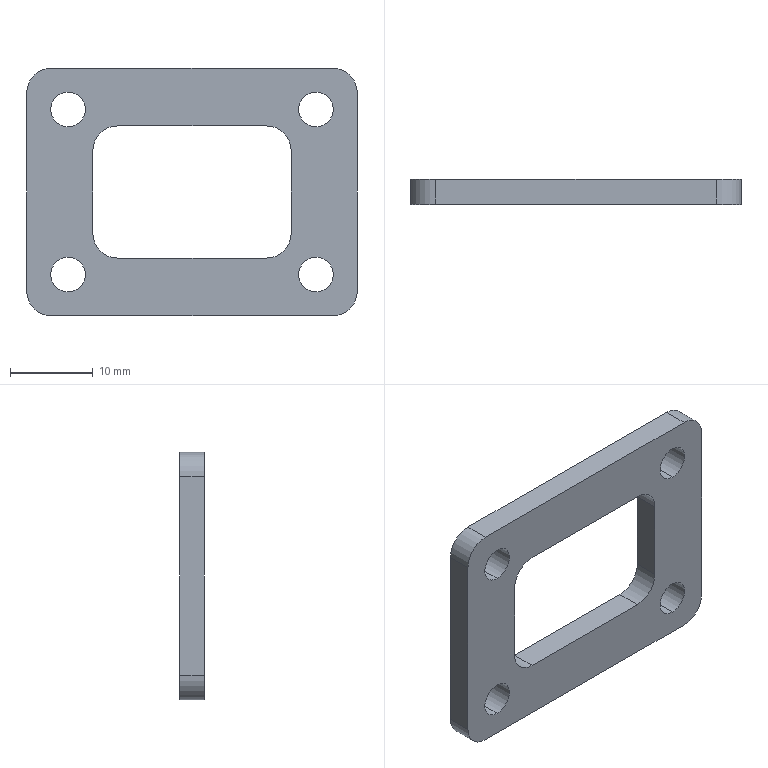Part | SolidWorks | features Extrusion 1 | 1 solid | 26 faces | box 40 x 3 x 30 mm | volume 2282 mm3 | cylinder 16 | plane 10 | commonest cylinder face diameters 4.2 x8 6 x8
STEP:
#1=CARTESIAN_POINT('',(15.,3.,7.9));
#2=VERTEX_POINT('',#1);
#3=CARTESIAN_POINT('',(15.,3.,12.1));
#4=VERTEX_POINT('',#3);
#5=CARTESIAN_POINT('',(15.,3.,10.));
#6=DIRECTION('',(0.,1.,0.));
#7=DIRECTION('',(0.,0.,1.));
#8=AXIS2_PLACEMENT_3D('',#5,#6,#7);
#9=CIRCLE('',#8,2.1);
#10=EDGE_CURVE('',#2,#4,#9,.T.);
#11=ORIENTED_EDGE('',*,*,#10,.T.);
#12=CARTESIAN_POINT('',(15.,0.,12.1));
#13=VERTEX_POINT('',#12);
#14=CARTESIAN_POINT('',(15.,3.,12.1));
#15=DIRECTION('',(0.,-1.,0.));
#16=VECTOR('',#15,1000.);
#17=LINE('',#14,#16);
#18=EDGE_CURVE('',#4,#13,#17,.T.);
#19=ORIENTED_EDGE('',*,*,#18,.T.);
#20=CARTESIAN_POINT('',(15.,0.,7.9));
#21=VERTEX_POINT('',#20);
#22=CARTESIAN_POINT('',(15.,0.,10.));
#23=DIRECTION('',(0.,1.,0.));
#24=DIRECTION('',(0.,0.,1.));
#25=AXIS2_PLACEMENT_3D('',#22,#23,#24);
#26=CIRCLE('',#25,2.1);
#27=EDGE_CURVE('',#21,#13,#26,.T.);
#28=ORIENTED_EDGE('',*,*,#27,.F.);
#29=CARTESIAN_POINT('',(15.,3.,7.9));
#30=DIRECTION('',(0.,-1.,0.));
#31=VECTOR('',#30,1000.);
#32=LINE('',#29,#31);
#33=EDGE_CURVE('',#2,#21,#32,.T.);
#34=ORIENTED_EDGE('',*,*,#33,.F.);
#35=EDGE_LOOP('',(#11,#19,#28,#34));
#36=FACE_OUTER_BOUND('',#35,.T.);
#37=CARTESIAN_POINT('',(15.,3.,10.));
#38=DIRECTION('',(0.,-1.,0.));
#39=DIRECTION('',(0.,0.,-1.));
#40=AXIS2_PLACEMENT_3D('',#37,#38,#39);
#41=CYLINDRICAL_SURFACE('',#40,2.1);
#42=ADVANCED_FACE('',(#36),#41,.F.);
#43=CARTESIAN_POINT('',(-15.,3.,7.9));
#44=VERTEX_POINT('',#43);
#45=CARTESIAN_POINT('',(-15.,3.,12.1));
#46=VERTEX_POINT('',#45);
#47=CARTESIAN_POINT('',(-15.,3.,10.));
#48=DIRECTION('',(0.,1.,0.));
#49=DIRECTION('',(0.,0.,1.));
#50=AXIS2_PLACEMENT_3D('',#47,#48,#49);
#51=CIRCLE('',#50,2.1);
#52=EDGE_CURVE('',#44,#46,#51,.T.);
#53=ORIENTED_EDGE('',*,*,#52,.T.);
#54=CARTESIAN_POINT('',(-15.,0.,12.1));
#55=VERTEX_POINT('',#54);
#56=CARTESIAN_POINT('',(-15.,3.,12.1));
#57=DIRECTION('',(0.,-1.,0.));
#58=VECTOR('',#57,1000.);
#59=LINE('',#56,#58);
#60=EDGE_CURVE('',#46,#55,#59,.T.);
#61=ORIENTED_EDGE('',*,*,#60,.T.);
#62=CARTESIAN_POINT('',(-15.,0.,7.9));
#63=VERTEX_POINT('',#62);
#64=CARTESIAN_POINT('',(-15.,0.,10.));
#65=DIRECTION('',(0.,1.,0.));
#66=DIRECTION('',(0.,0.,1.));
#67=AXIS2_PLACEMENT_3D('',#64,#65,#66);
#68=CIRCLE('',#67,2.1);
#69=EDGE_CURVE('',#63,#55,#68,.T.);
#70=ORIENTED_EDGE('',*,*,#69,.F.);
#71=CARTESIAN_POINT('',(-15.,3.,7.9));
#72=DIRECTION('',(0.,-1.,0.));
#73=VECTOR('',#72,1000.);
#74=LINE('',#71,#73);
#75=EDGE_CURVE('',#44,#63,#74,.T.);
#76=ORIENTED_EDGE('',*,*,#75,.F.);
#77=EDGE_LOOP('',(#53,#61,#70,#76));
#78=FACE_OUTER_BOUND('',#77,.T.);
#79=CARTESIAN_POINT('',(-15.,3.,10.));
#80=DIRECTION('',(0.,-1.,0.));
#81=DIRECTION('',(0.,0.,-1.));
#82=AXIS2_PLACEMENT_3D('',#79,#80,#81);
#83=CYLINDRICAL_SURFACE('',#82,2.1);
#84=ADVANCED_FACE('',(#78),#83,.F.);
#85=CARTESIAN_POINT('',(15.,3.,-12.1));
#86=VERTEX_POINT('',#85);
#87=CARTESIAN_POINT('',(15.,3.,-7.9));
#88=VERTEX_POINT('',#87);
#89=CARTESIAN_POINT('',(15.,3.,-10.));
#90=DIRECTION('',(0.,1.,0.));
#91=DIRECTION('',(0.,0.,1.));
#92=AXIS2_PLACEMENT_3D('',#89,#90,#91);
#93=CIRCLE('',#92,2.1);
#94=EDGE_CURVE('',#86,#88,#93,.T.);
#95=ORIENTED_EDGE('',*,*,#94,.T.);
#96=CARTESIAN_POINT('',(15.,0.,-7.9));
#97=VERTEX_POINT('',#96);
#98=CARTESIAN_POINT('',(15.,3.,-7.9));
#99=DIRECTION('',(0.,-1.,0.));
#100=VECTOR('',#99,1000.);
#101=LINE('',#98,#100);
#102=EDGE_CURVE('',#88,#97,#101,.T.);
#103=ORIENTED_EDGE('',*,*,#102,.T.);
#104=CARTESIAN_POINT('',(15.,0.,-12.1));
#105=VERTEX_POINT('',#104);
#106=CARTESIAN_POINT('',(15.,0.,-10.));
#107=DIRECTION('',(0.,1.,0.));
#108=DIRECTION('',(0.,0.,1.));
#109=AXIS2_PLACEMENT_3D('',#106,#107,#108);
#110=CIRCLE('',#109,2.1);
#111=EDGE_CURVE('',#105,#97,#110,.T.);
#112=ORIENTED_EDGE('',*,*,#111,.F.);
#113=CARTESIAN_POINT('',(15.,3.,-12.1));
#114=DIRECTION('',(0.,-1.,0.));
#115=VECTOR('',#114,1000.);
#116=LINE('',#113,#115);
#117=EDGE_CURVE('',#86,#105,#116,.T.);
#118=ORIENTED_EDGE('',*,*,#117,.F.);
#119=EDGE_LOOP('',(#95,#103,#112,#118));
#120=FACE_OUTER_BOUND('',#119,.T.);
#121=CARTESIAN_POINT('',(15.,3.,-10.));
#122=DIRECTION('',(0.,-1.,0.));
#123=DIRECTION('',(0.,0.,-1.));
#124=AXIS2_PLACEMENT_3D('',#121,#122,#123);
#125=CYLINDRICAL_SURFACE('',#124,2.1);
#126=ADVANCED_FACE('',(#120),#125,.F.);
#127=CARTESIAN_POINT('',(-15.,3.,-12.1));
#128=VERTEX_POINT('',#127);
#129=CARTESIAN_POINT('',(-15.,3.,-7.9));
#130=VERTEX_POINT('',#129);
#131=CARTESIAN_POINT('',(-15.,3.,-10.));
#132=DIRECTION('',(0.,1.,0.));
#133=DIRECTION('',(0.,0.,1.));
#134=AXIS2_PLACEMENT_3D('',#131,#132,#133);
#135=CIRCLE('',#134,2.1);
#136=EDGE_CURVE('',#128,#130,#135,.T.);
#137=ORIENTED_EDGE('',*,*,#136,.T.);
#138=CARTESIAN_POINT('',(-15.,0.,-7.9));
#139=VERTEX_POINT('',#138);
#140=CARTESIAN_POINT('',(-15.,3.,-7.9));
#141=DIRECTION('',(0.,-1.,0.));
#142=VECTOR('',#141,1000.);
#143=LINE('',#140,#142);
#144=EDGE_CURVE('',#130,#139,#143,.T.);
#145=ORIENTED_EDGE('',*,*,#144,.T.);
#146=CARTESIAN_POINT('',(-15.,0.,-12.1));
#147=VERTEX_POINT('',#146);
#148=CARTESIAN_POINT('',(-15.,0.,-10.));
#149=DIRECTION('',(0.,1.,0.));
#150=DIRECTION('',(0.,0.,1.));
#151=AXIS2_PLACEMENT_3D('',#148,#149,#150);
#152=CIRCLE('',#151,2.1);
#153=EDGE_CURVE('',#147,#139,#152,.T.);
#154=ORIENTED_EDGE('',*,*,#153,.F.);
#155=CARTESIAN_POINT('',(-15.,3.,-12.1));
#156=DIRECTION('',(0.,-1.,0.));
#157=VECTOR('',#156,1000.);
#158=LINE('',#155,#157);
#159=EDGE_CURVE('',#128,#147,#158,.T.);
#160=ORIENTED_EDGE('',*,*,#159,.F.);
#161=EDGE_LOOP('',(#137,#145,#154,#160));
#162=FACE_OUTER_BOUND('',#161,.T.);
#163=CARTESIAN_POINT('',(-15.,3.,-10.));
#164=DIRECTION('',(0.,-1.,0.));
#165=DIRECTION('',(0.,0.,-1.));
#166=AXIS2_PLACEMENT_3D('',#163,#164,#165);
#167=CYLINDRICAL_SURFACE('',#166,2.1);
#168=ADVANCED_FACE('',(#162),#167,.F.);
#169=ORIENTED_EDGE('',*,*,#52,.F.);
#170=CARTESIAN_POINT('',(-15.,3.,10.));
#171=DIRECTION('',(0.,1.,0.));
#172=DIRECTION('',(0.,0.,1.));
#173=AXIS2_PLACEMENT_3D('',#170,#171,#172);
#174=CIRCLE('',#173,2.1);
#175=EDGE_CURVE('',#46,#44,#174,.T.);
#176=ORIENTED_EDGE('',*,*,#175,.F.);
#177=EDGE_LOOP('',(#169,#176));
#178=FACE_BOUND('',#177,.T.);
#179=ORIENTED_EDGE('',*,*,#136,.F.);
#180=CARTESIAN_POINT('',(-15.,3.,-10.));
#181=DIRECTION('',(0.,1.,0.));
#182=DIRECTION('',(0.,0.,1.));
#183=AXIS2_PLACEMENT_3D('',#180,#181,#182);
#184=CIRCLE('',#183,2.1);
#185=EDGE_CURVE('',#130,#128,#184,.T.);
#186=ORIENTED_EDGE('',*,*,#185,.F.);
#187=EDGE_LOOP('',(#179,#186));
#188=FACE_BOUND('',#187,.T.);
#189=CARTESIAN_POINT('',(17.,3.,15.));
#190=VERTEX_POINT('',#189);
#191=CARTESIAN_POINT('',(20.,3.,12.));
#192=VERTEX_POINT('',#191);
#193=CARTESIAN_POINT('',(17.,3.,12.));
#194=DIRECTION('',(0.,1.,0.));
#195=DIRECTION('',(0.,0.,1.));
#196=AXIS2_PLACEMENT_3D('',#193,#194,#195);
#197=CIRCLE('',#196,3.);
#198=EDGE_CURVE('',#190,#192,#197,.T.);
#199=ORIENTED_EDGE('',*,*,#198,.T.);
#200=CARTESIAN_POINT('',(20.,3.,-12.));
#201=VERTEX_POINT('',#200);
#202=CARTESIAN_POINT('',(20.,3.,12.));
#203=DIRECTION('',(0.,0.,-1.));
#204=VECTOR('',#203,1000.);
#205=LINE('',#202,#204);
#206=EDGE_CURVE('',#192,#201,#205,.T.);
#207=ORIENTED_EDGE('',*,*,#206,.T.);
#208=CARTESIAN_POINT('',(17.,3.,-15.));
#209=VERTEX_POINT('',#208);
#210=CARTESIAN_POINT('',(17.,3.,-12.));
#211=DIRECTION('',(0.,1.,0.));
#212=DIRECTION('',(0.,0.,-1.));
#213=AXIS2_PLACEMENT_3D('',#210,#211,#212);
#214=CIRCLE('',#213,3.);
#215=EDGE_CURVE('',#201,#209,#214,.T.);
#216=ORIENTED_EDGE('',*,*,#215,.T.);
#217=CARTESIAN_POINT('',(-17.,3.,-15.));
#218=VERTEX_POINT('',#217);
#219=CARTESIAN_POINT('',(-17.,3.,-15.));
#220=DIRECTION('',(-1.,0.,0.));
#221=VECTOR('',#220,1000.);
#222=LINE('',#219,#221);
#223=EDGE_CURVE('',#209,#218,#222,.T.);
#224=ORIENTED_EDGE('',*,*,#223,.T.);
#225=CARTESIAN_POINT('',(-20.,3.,-12.));
#226=VERTEX_POINT('',#225);
#227=CARTESIAN_POINT('',(-17.,3.,-12.));
#228=DIRECTION('',(0.,1.,0.));
#229=DIRECTION('',(0.,0.,-1.));
#230=AXIS2_PLACEMENT_3D('',#227,#228,#229);
#231=CIRCLE('',#230,3.);
#232=EDGE_CURVE('',#218,#226,#231,.T.);
#233=ORIENTED_EDGE('',*,*,#232,.T.);
#234=CARTESIAN_POINT('',(-20.,3.,12.));
#235=VERTEX_POINT('',#234);
#236=CARTESIAN_POINT('',(-20.,3.,12.));
#237=DIRECTION('',(0.,0.,1.));
#238=VECTOR('',#237,1000.);
#239=LINE('',#236,#238);
#240=EDGE_CURVE('',#226,#235,#239,.T.);
#241=ORIENTED_EDGE('',*,*,#240,.T.);
#242=CARTESIAN_POINT('',(-17.,3.,15.));
#243=VERTEX_POINT('',#242);
#244=CARTESIAN_POINT('',(-17.,3.,12.));
#245=DIRECTION('',(0.,1.,0.));
#246=DIRECTION('',(0.,0.,-1.));
#247=AXIS2_PLACEMENT_3D('',#244,#245,#246);
#248=CIRCLE('',#247,3.);
#249=EDGE_CURVE('',#235,#243,#248,.T.);
#250=ORIENTED_EDGE('',*,*,#249,.T.);
#251=CARTESIAN_POINT('',(-17.,3.,15.));
#252=DIRECTION('',(1.,0.,0.));
#253=VECTOR('',#252,1000.);
#254=LINE('',#251,#253);
#255=EDGE_CURVE('',#243,#190,#254,.T.);
#256=ORIENTED_EDGE('',*,*,#255,.T.);
#257=EDGE_LOOP('',(#199,#207,#216,#224,#233,#241,#250,#256));
#258=FACE_OUTER_BOUND('',#257,.T.);
#259=ORIENTED_EDGE('',*,*,#94,.F.);
#260=CARTESIAN_POINT('',(15.,3.,-10.));
#261=DIRECTION('',(0.,1.,0.));
#262=DIRECTION('',(0.,0.,1.));
#263=AXIS2_PLACEMENT_3D('',#260,#261,#262);
#264=CIRCLE('',#263,2.1);
#265=EDGE_CURVE('',#88,#86,#264,.T.);
#266=ORIENTED_EDGE('',*,*,#265,.F.);
#267=EDGE_LOOP('',(#259,#266));
#268=FACE_BOUND('',#267,.T.);
#269=ORIENTED_EDGE('',*,*,#10,.F.);
#270=CARTESIAN_POINT('',(15.,3.,10.));
#271=DIRECTION('',(0.,1.,0.));
#272=DIRECTION('',(0.,0.,1.));
#273=AXIS2_PLACEMENT_3D('',#270,#271,#272);
#274=CIRCLE('',#273,2.1);
#275=EDGE_CURVE('',#4,#2,#274,.T.);
#276=ORIENTED_EDGE('',*,*,#275,.F.);
#277=EDGE_LOOP('',(#269,#276));
#278=FACE_BOUND('',#277,.T.);
#279=CARTESIAN_POINT('',(12.,3.,5.));
#280=VERTEX_POINT('',#279);
#281=CARTESIAN_POINT('',(12.,3.,-5.));
#282=VERTEX_POINT('',#281);
#283=CARTESIAN_POINT('',(12.,3.,5.));
#284=DIRECTION('',(0.,0.,-1.));
#285=VECTOR('',#284,1000.);
#286=LINE('',#283,#285);
#287=EDGE_CURVE('',#280,#282,#286,.T.);
#288=ORIENTED_EDGE('',*,*,#287,.F.);
#289=CARTESIAN_POINT('',(9.,3.,8.));
#290=VERTEX_POINT('',#289);
#291=CARTESIAN_POINT('',(9.,3.,5.));
#292=DIRECTION('',(0.,1.,0.));
#293=DIRECTION('',(0.,0.,1.));
#294=AXIS2_PLACEMENT_3D('',#291,#292,#293);
#295=CIRCLE('',#294,3.);
#296=EDGE_CURVE('',#290,#280,#295,.T.);
#297=ORIENTED_EDGE('',*,*,#296,.F.);
#298=CARTESIAN_POINT('',(-9.,3.,8.));
#299=VERTEX_POINT('',#298);
#300=CARTESIAN_POINT('',(-9.,3.,8.));
#301=DIRECTION('',(1.,0.,0.));
#302=VECTOR('',#301,1000.);
#303=LINE('',#300,#302);
#304=EDGE_CURVE('',#299,#290,#303,.T.);
#305=ORIENTED_EDGE('',*,*,#304,.F.);
#306=CARTESIAN_POINT('',(-12.,3.,5.));
#307=VERTEX_POINT('',#306);
#308=CARTESIAN_POINT('',(-9.,3.,5.));
#309=DIRECTION('',(0.,1.,0.));
#310=DIRECTION('',(0.,0.,-1.));
#311=AXIS2_PLACEMENT_3D('',#308,#309,#310);
#312=CIRCLE('',#311,3.);
#313=EDGE_CURVE('',#307,#299,#312,.T.);
#314=ORIENTED_EDGE('',*,*,#313,.F.);
#315=CARTESIAN_POINT('',(-12.,3.,-5.));
#316=VERTEX_POINT('',#315);
#317=CARTESIAN_POINT('',(-12.,3.,5.));
#318=DIRECTION('',(0.,0.,1.));
#319=VECTOR('',#318,1000.);
#320=LINE('',#317,#319);
#321=EDGE_CURVE('',#316,#307,#320,.T.);
#322=ORIENTED_EDGE('',*,*,#321,.F.);
#323=CARTESIAN_POINT('',(-9.,3.,-8.));
#324=VERTEX_POINT('',#323);
#325=CARTESIAN_POINT('',(-9.,3.,-5.));
#326=DIRECTION('',(0.,1.,0.));
#327=DIRECTION('',(0.,0.,-1.));
#328=AXIS2_PLACEMENT_3D('',#325,#326,#327);
#329=CIRCLE('',#328,3.);
#330=EDGE_CURVE('',#324,#316,#329,.T.);
#331=ORIENTED_EDGE('',*,*,#330,.F.);
#332=CARTESIAN_POINT('',(9.,3.,-8.));
#333=VERTEX_POINT('',#332);
#334=CARTESIAN_POINT('',(-9.,3.,-8.));
#335=DIRECTION('',(-1.,0.,0.));
#336=VECTOR('',#335,1000.);
#337=LINE('',#334,#336);
#338=EDGE_CURVE('',#333,#324,#337,.T.);
#339=ORIENTED_EDGE('',*,*,#338,.F.);
#340=CARTESIAN_POINT('',(9.,3.,-5.));
#341=DIRECTION('',(0.,1.,0.));
#342=DIRECTION('',(0.,0.,-1.));
#343=AXIS2_PLACEMENT_3D('',#340,#341,#342);
#344=CIRCLE('',#343,3.);
#345=EDGE_CURVE('',#282,#333,#344,.T.);
#346=ORIENTED_EDGE('',*,*,#345,.F.);
#347=EDGE_LOOP('',(#288,#297,#305,#314,#322,#331,#339,#346));
#348=FACE_BOUND('',#347,.T.);
#349=CARTESIAN_POINT('',(17.,3.,12.));
#350=DIRECTION('',(0.,1.,0.));
#351=DIRECTION('',(0.,0.,1.));
#352=AXIS2_PLACEMENT_3D('',#349,#350,#351);
#353=PLANE('',#352);
#354=ADVANCED_FACE('',(#178,#188,#258,#268,#278,#348),#353,.T.);
#355=ORIENTED_EDGE('',*,*,#27,.T.);
#356=CARTESIAN_POINT('',(15.,0.,10.));
#357=DIRECTION('',(0.,1.,0.));
#358=DIRECTION('',(0.,0.,1.));
#359=AXIS2_PLACEMENT_3D('',#356,#357,#358);
#360=CIRCLE('',#359,2.1);
#361=EDGE_CURVE('',#13,#21,#360,.T.);
#362=ORIENTED_EDGE('',*,*,#361,.T.);
#363=EDGE_LOOP('',(#355,#362));
#364=FACE_BOUND('',#363,.T.);
#365=ORIENTED_EDGE('',*,*,#69,.T.);
#366=CARTESIAN_POINT('',(-15.,0.,10.));
#367=DIRECTION('',(0.,1.,0.));
#368=DIRECTION('',(0.,0.,1.));
#369=AXIS2_PLACEMENT_3D('',#366,#367,#368);
#370=CIRCLE('',#369,2.1);
#371=EDGE_CURVE('',#55,#63,#370,.T.);
#372=ORIENTED_EDGE('',*,*,#371,.T.);
#373=EDGE_LOOP('',(#365,#372));
#374=FACE_BOUND('',#373,.T.);
#375=ORIENTED_EDGE('',*,*,#111,.T.);
#376=CARTESIAN_POINT('',(15.,0.,-10.));
#377=DIRECTION('',(0.,1.,0.));
#378=DIRECTION('',(0.,0.,1.));
#379=AXIS2_PLACEMENT_3D('',#376,#377,#378);
#380=CIRCLE('',#379,2.1);
#381=EDGE_CURVE('',#97,#105,#380,.T.);
#382=ORIENTED_EDGE('',*,*,#381,.T.);
#383=EDGE_LOOP('',(#375,#382));
#384=FACE_BOUND('',#383,.T.);
#385=ORIENTED_EDGE('',*,*,#153,.T.);
#386=CARTESIAN_POINT('',(-15.,0.,-10.));
#387=DIRECTION('',(0.,1.,0.));
#388=DIRECTION('',(0.,0.,1.));
#389=AXIS2_PLACEMENT_3D('',#386,#387,#388);
#390=CIRCLE('',#389,2.1);
#391=EDGE_CURVE('',#139,#147,#390,.T.);
#392=ORIENTED_EDGE('',*,*,#391,.T.);
#393=EDGE_LOOP('',(#385,#392));
#394=FACE_BOUND('',#393,.T.);
#395=CARTESIAN_POINT('',(17.,0.,15.));
#396=VERTEX_POINT('',#395);
#397=CARTESIAN_POINT('',(20.,0.,12.));
#398=VERTEX_POINT('',#397);
#399=CARTESIAN_POINT('',(17.,0.,12.));
#400=DIRECTION('',(0.,1.,0.));
#401=DIRECTION('',(0.,0.,1.));
#402=AXIS2_PLACEMENT_3D('',#399,#400,#401);
#403=CIRCLE('',#402,3.);
#404=EDGE_CURVE('',#396,#398,#403,.T.);
#405=ORIENTED_EDGE('',*,*,#404,.F.);
#406=CARTESIAN_POINT('',(-17.,0.,15.));
#407=VERTEX_POINT('',#406);
#408=CARTESIAN_POINT('',(-17.,0.,15.));
#409=DIRECTION('',(1.,0.,0.));
#410=VECTOR('',#409,1000.);
#411=LINE('',#408,#410);
#412=EDGE_CURVE('',#407,#396,#411,.T.);
#413=ORIENTED_EDGE('',*,*,#412,.F.);
#414=CARTESIAN_POINT('',(-20.,0.,12.));
#415=VERTEX_POINT('',#414);
#416=CARTESIAN_POINT('',(-17.,0.,12.));
#417=DIRECTION('',(0.,1.,0.));
#418=DIRECTION('',(0.,0.,-1.));
#419=AXIS2_PLACEMENT_3D('',#416,#417,#418);
#420=CIRCLE('',#419,3.);
#421=EDGE_CURVE('',#415,#407,#420,.T.);
#422=ORIENTED_EDGE('',*,*,#421,.F.);
#423=CARTESIAN_POINT('',(-20.,0.,-12.));
#424=VERTEX_POINT('',#423);
#425=CARTESIAN_POINT('',(-20.,0.,12.));
#426=DIRECTION('',(0.,0.,1.));
#427=VECTOR('',#426,1000.);
#428=LINE('',#425,#427);
#429=EDGE_CURVE('',#424,#415,#428,.T.);
#430=ORIENTED_EDGE('',*,*,#429,.F.);
#431=CARTESIAN_POINT('',(-17.,0.,-15.));
#432=VERTEX_POINT('',#431);
#433=CARTESIAN_POINT('',(-17.,0.,-12.));
#434=DIRECTION('',(0.,1.,0.));
#435=DIRECTION('',(0.,0.,-1.));
#436=AXIS2_PLACEMENT_3D('',#433,#434,#435);
#437=CIRCLE('',#436,3.);
#438=EDGE_CURVE('',#432,#424,#437,.T.);
#439=ORIENTED_EDGE('',*,*,#438,.F.);
#440=CARTESIAN_POINT('',(17.,0.,-15.));
#441=VERTEX_POINT('',#440);
#442=CARTESIAN_POINT('',(-17.,0.,-15.));
#443=DIRECTION('',(-1.,0.,0.));
#444=VECTOR('',#443,1000.);
#445=LINE('',#442,#444);
#446=EDGE_CURVE('',#441,#432,#445,.T.);
#447=ORIENTED_EDGE('',*,*,#446,.F.);
#448=CARTESIAN_POINT('',(20.,0.,-12.));
#449=VERTEX_POINT('',#448);
#450=CARTESIAN_POINT('',(17.,0.,-12.));
#451=DIRECTION('',(0.,1.,0.));
#452=DIRECTION('',(0.,0.,-1.));
#453=AXIS2_PLACEMENT_3D('',#450,#451,#452);
#454=CIRCLE('',#453,3.);
#455=EDGE_CURVE('',#449,#441,#454,.T.);
#456=ORIENTED_EDGE('',*,*,#455,.F.);
#457=CARTESIAN_POINT('',(20.,0.,12.));
#458=DIRECTION('',(0.,0.,-1.));
#459=VECTOR('',#458,1000.);
#460=LINE('',#457,#459);
#461=EDGE_CURVE('',#398,#449,#460,.T.);
#462=ORIENTED_EDGE('',*,*,#461,.F.);
#463=EDGE_LOOP('',(#405,#413,#422,#430,#439,#447,#456,#462));
#464=FACE_OUTER_BOUND('',#463,.T.);
#465=CARTESIAN_POINT('',(9.,0.,8.));
#466=VERTEX_POINT('',#465);
#467=CARTESIAN_POINT('',(12.,0.,5.));
#468=VERTEX_POINT('',#467);
#469=CARTESIAN_POINT('',(9.,0.,5.));
#470=DIRECTION('',(0.,1.,0.));
#471=DIRECTION('',(0.,0.,1.));
#472=AXIS2_PLACEMENT_3D('',#469,#470,#471);
#473=CIRCLE('',#472,3.);
#474=EDGE_CURVE('',#466,#468,#473,.T.);
#475=ORIENTED_EDGE('',*,*,#474,.T.);
#476=CARTESIAN_POINT('',(12.,0.,-5.));
#477=VERTEX_POINT('',#476);
#478=CARTESIAN_POINT('',(12.,0.,5.));
#479=DIRECTION('',(0.,0.,-1.));
#480=VECTOR('',#479,1000.);
#481=LINE('',#478,#480);
#482=EDGE_CURVE('',#468,#477,#481,.T.);
#483=ORIENTED_EDGE('',*,*,#482,.T.);
#484=CARTESIAN_POINT('',(9.,0.,-8.));
#485=VERTEX_POINT('',#484);
#486=CARTESIAN_POINT('',(9.,0.,-5.));
#487=DIRECTION('',(0.,1.,0.));
#488=DIRECTION('',(0.,0.,-1.));
#489=AXIS2_PLACEMENT_3D('',#486,#487,#488);
#490=CIRCLE('',#489,3.);
#491=EDGE_CURVE('',#477,#485,#490,.T.);
#492=ORIENTED_EDGE('',*,*,#491,.T.);
#493=CARTESIAN_POINT('',(-9.,0.,-8.));
#494=VERTEX_POINT('',#493);
#495=CARTESIAN_POINT('',(-9.,0.,-8.));
#496=DIRECTION('',(-1.,0.,0.));
#497=VECTOR('',#496,1000.);
#498=LINE('',#495,#497);
#499=EDGE_CURVE('',#485,#494,#498,.T.);
#500=ORIENTED_EDGE('',*,*,#499,.T.);
#501=CARTESIAN_POINT('',(-12.,0.,-5.));
#502=VERTEX_POINT('',#501);
#503=CARTESIAN_POINT('',(-9.,0.,-5.));
#504=DIRECTION('',(0.,1.,0.));
#505=DIRECTION('',(0.,0.,-1.));
#506=AXIS2_PLACEMENT_3D('',#503,#504,#505);
#507=CIRCLE('',#506,3.);
#508=EDGE_CURVE('',#494,#502,#507,.T.);
#509=ORIENTED_EDGE('',*,*,#508,.T.);
#510=CARTESIAN_POINT('',(-12.,0.,5.));
#511=VERTEX_POINT('',#510);
#512=CARTESIAN_POINT('',(-12.,0.,5.));
#513=DIRECTION('',(0.,0.,1.));
#514=VECTOR('',#513,1000.);
#515=LINE('',#512,#514);
#516=EDGE_CURVE('',#502,#511,#515,.T.);
#517=ORIENTED_EDGE('',*,*,#516,.T.);
#518=CARTESIAN_POINT('',(-9.,0.,8.));
#519=VERTEX_POINT('',#518);
#520=CARTESIAN_POINT('',(-9.,0.,5.));
#521=DIRECTION('',(0.,1.,0.));
#522=DIRECTION('',(0.,0.,-1.));
#523=AXIS2_PLACEMENT_3D('',#520,#521,#522);
#524=CIRCLE('',#523,3.);
#525=EDGE_CURVE('',#511,#519,#524,.T.);
#526=ORIENTED_EDGE('',*,*,#525,.T.);
#527=CARTESIAN_POINT('',(-9.,0.,8.));
#528=DIRECTION('',(1.,0.,0.));
#529=VECTOR('',#528,1000.);
#530=LINE('',#527,#529);
#531=EDGE_CURVE('',#519,#466,#530,.T.);
#532=ORIENTED_EDGE('',*,*,#531,.T.);
#533=EDGE_LOOP('',(#475,#483,#492,#500,#509,#517,#526,#532));
#534=FACE_BOUND('',#533,.T.);
#535=CARTESIAN_POINT('',(17.,0.,12.));
#536=DIRECTION('',(0.,1.,0.));
#537=DIRECTION('',(0.,0.,1.));
#538=AXIS2_PLACEMENT_3D('',#535,#536,#537);
#539=PLANE('',#538);
#540=ADVANCED_FACE('',(#364,#374,#384,#394,#464,#534),#539,.F.);
#541=ORIENTED_EDGE('',*,*,#404,.T.);
#542=CARTESIAN_POINT('',(20.,3.,12.));
#543=DIRECTION('',(0.,-1.,0.));
#544=VECTOR('',#543,1000.);
#545=LINE('',#542,#544);
#546=EDGE_CURVE('',#192,#398,#545,.T.);
#547=ORIENTED_EDGE('',*,*,#546,.F.);
#548=ORIENTED_EDGE('',*,*,#198,.F.);
#549=CARTESIAN_POINT('',(17.,3.,15.));
#550=DIRECTION('',(0.,-1.,0.));
#551=VECTOR('',#550,1000.);
#552=LINE('',#549,#551);
#553=EDGE_CURVE('',#190,#396,#552,.T.);
#554=ORIENTED_EDGE('',*,*,#553,.T.);
#555=EDGE_LOOP('',(#541,#547,#548,#554));
#556=FACE_OUTER_BOUND('',#555,.T.);
#557=CARTESIAN_POINT('',(17.,3.,12.));
#558=DIRECTION('',(0.,-1.,0.));
#559=DIRECTION('',(0.,0.,-1.));
#560=AXIS2_PLACEMENT_3D('',#557,#558,#559);
#561=CYLINDRICAL_SURFACE('',#560,3.);
#562=ADVANCED_FACE('',(#556),#561,.T.);
#563=ORIENTED_EDGE('',*,*,#461,.T.);
#564=CARTESIAN_POINT('',(20.,3.,-12.));
#565=DIRECTION('',(0.,-1.,0.));
#566=VECTOR('',#565,1000.);
#567=LINE('',#564,#566);
#568=EDGE_CURVE('',#201,#449,#567,.T.);
#569=ORIENTED_EDGE('',*,*,#568,.F.);
#570=ORIENTED_EDGE('',*,*,#206,.F.);
#571=ORIENTED_EDGE('',*,*,#546,.T.);
#572=EDGE_LOOP('',(#563,#569,#570,#571));
#573=FACE_OUTER_BOUND('',#572,.T.);
#574=CARTESIAN_POINT('',(20.,3.,12.));
#575=DIRECTION('',(-1.,0.,0.));
#576=DIRECTION('',(0.,0.,1.));
#577=AXIS2_PLACEMENT_3D('',#574,#575,#576);
#578=PLANE('',#577);
#579=ADVANCED_FACE('',(#573),#578,.F.);
#580=ORIENTED_EDGE('',*,*,#455,.T.);
#581=CARTESIAN_POINT('',(17.,3.,-15.));
#582=DIRECTION('',(0.,-1.,0.));
#583=VECTOR('',#582,1000.);
#584=LINE('',#581,#583);
#585=EDGE_CURVE('',#209,#441,#584,.T.);
#586=ORIENTED_EDGE('',*,*,#585,.F.);
#587=ORIENTED_EDGE('',*,*,#215,.F.);
#588=ORIENTED_EDGE('',*,*,#568,.T.);
#589=EDGE_LOOP('',(#580,#586,#587,#588));
#590=FACE_OUTER_BOUND('',#589,.T.);
#591=CARTESIAN_POINT('',(17.,3.,-12.));
#592=DIRECTION('',(0.,-1.,0.));
#593=DIRECTION('',(0.,0.,-1.));
#594=AXIS2_PLACEMENT_3D('',#591,#592,#593);
#595=CYLINDRICAL_SURFACE('',#594,3.);
#596=ADVANCED_FACE('',(#590),#595,.T.);
#597=ORIENTED_EDGE('',*,*,#446,.T.);
#598=CARTESIAN_POINT('',(-17.,3.,-15.));
#599=DIRECTION('',(0.,-1.,0.));
#600=VECTOR('',#599,1000.);
#601=LINE('',#598,#600);
#602=EDGE_CURVE('',#218,#432,#601,.T.);
#603=ORIENTED_EDGE('',*,*,#602,.F.);
#604=ORIENTED_EDGE('',*,*,#223,.F.);
#605=ORIENTED_EDGE('',*,*,#585,.T.);
#606=EDGE_LOOP('',(#597,#603,#604,#605));
#607=FACE_OUTER_BOUND('',#606,.T.);
#608=CARTESIAN_POINT('',(-17.,3.,-15.));
#609=DIRECTION('',(0.,0.,1.));
#610=DIRECTION('',(1.,0.,0.));
#611=AXIS2_PLACEMENT_3D('',#608,#609,#610);
#612=PLANE('',#611);
#613=ADVANCED_FACE('',(#607),#612,.F.);
#614=ORIENTED_EDGE('',*,*,#438,.T.);
#615=CARTESIAN_POINT('',(-20.,3.,-12.));
#616=DIRECTION('',(0.,-1.,0.));
#617=VECTOR('',#616,1000.);
#618=LINE('',#615,#617);
#619=EDGE_CURVE('',#226,#424,#618,.T.);
#620=ORIENTED_EDGE('',*,*,#619,.F.);
#621=ORIENTED_EDGE('',*,*,#232,.F.);
#622=ORIENTED_EDGE('',*,*,#602,.T.);
#623=EDGE_LOOP('',(#614,#620,#621,#622));
#624=FACE_OUTER_BOUND('',#623,.T.);
#625=CARTESIAN_POINT('',(-17.,3.,-12.));
#626=DIRECTION('',(0.,-1.,0.));
#627=DIRECTION('',(0.,0.,-1.));
#628=AXIS2_PLACEMENT_3D('',#625,#626,#627);
#629=CYLINDRICAL_SURFACE('',#628,3.);
#630=ADVANCED_FACE('',(#624),#629,.T.);
#631=ORIENTED_EDGE('',*,*,#429,.T.);
#632=CARTESIAN_POINT('',(-20.,3.,12.));
#633=DIRECTION('',(0.,-1.,0.));
#634=VECTOR('',#633,1000.);
#635=LINE('',#632,#634);
#636=EDGE_CURVE('',#235,#415,#635,.T.);
#637=ORIENTED_EDGE('',*,*,#636,.F.);
#638=ORIENTED_EDGE('',*,*,#240,.F.);
#639=ORIENTED_EDGE('',*,*,#619,.T.);
#640=EDGE_LOOP('',(#631,#637,#638,#639));
#641=FACE_OUTER_BOUND('',#640,.T.);
#642=CARTESIAN_POINT('',(-20.,3.,12.));
#643=DIRECTION('',(1.,0.,0.));
#644=DIRECTION('',(0.,0.,-1.));
#645=AXIS2_PLACEMENT_3D('',#642,#643,#644);
#646=PLANE('',#645);
#647=ADVANCED_FACE('',(#641),#646,.F.);
#648=ORIENTED_EDGE('',*,*,#421,.T.);
#649=CARTESIAN_POINT('',(-17.,3.,15.));
#650=DIRECTION('',(0.,-1.,0.));
#651=VECTOR('',#650,1000.);
#652=LINE('',#649,#651);
#653=EDGE_CURVE('',#243,#407,#652,.T.);
#654=ORIENTED_EDGE('',*,*,#653,.F.);
#655=ORIENTED_EDGE('',*,*,#249,.F.);
#656=ORIENTED_EDGE('',*,*,#636,.T.);
#657=EDGE_LOOP('',(#648,#654,#655,#656));
#658=FACE_OUTER_BOUND('',#657,.T.);
#659=CARTESIAN_POINT('',(-17.,3.,12.));
#660=DIRECTION('',(0.,-1.,0.));
#661=DIRECTION('',(0.,0.,-1.));
#662=AXIS2_PLACEMENT_3D('',#659,#660,#661);
#663=CYLINDRICAL_SURFACE('',#662,3.);
#664=ADVANCED_FACE('',(#658),#663,.T.);
#665=ORIENTED_EDGE('',*,*,#412,.T.);
#666=ORIENTED_EDGE('',*,*,#553,.F.);
#667=ORIENTED_EDGE('',*,*,#255,.F.);
#668=ORIENTED_EDGE('',*,*,#653,.T.);
#669=EDGE_LOOP('',(#665,#666,#667,#668));
#670=FACE_OUTER_BOUND('',#669,.T.);
#671=CARTESIAN_POINT('',(-17.,3.,15.));
#672=DIRECTION('',(0.,0.,-1.));
#673=DIRECTION('',(-1.,0.,0.));
#674=AXIS2_PLACEMENT_3D('',#671,#672,#673);
#675=PLANE('',#674);
#676=ADVANCED_FACE('',(#670),#675,.F.);
#677=ORIENTED_EDGE('',*,*,#144,.F.);
#678=ORIENTED_EDGE('',*,*,#185,.T.);
#679=ORIENTED_EDGE('',*,*,#159,.T.);
#680=ORIENTED_EDGE('',*,*,#391,.F.);
#681=EDGE_LOOP('',(#677,#678,#679,#680));
#682=FACE_OUTER_BOUND('',#681,.T.);
#683=CARTESIAN_POINT('',(-15.,3.,-10.));
#684=DIRECTION('',(0.,-1.,0.));
#685=DIRECTION('',(0.,0.,-1.));
#686=AXIS2_PLACEMENT_3D('',#683,#684,#685);
#687=CYLINDRICAL_SURFACE('',#686,2.1);
#688=ADVANCED_FACE('',(#682),#687,.F.);
#689=ORIENTED_EDGE('',*,*,#102,.F.);
#690=ORIENTED_EDGE('',*,*,#265,.T.);
#691=ORIENTED_EDGE('',*,*,#117,.T.);
#692=ORIENTED_EDGE('',*,*,#381,.F.);
#693=EDGE_LOOP('',(#689,#690,#691,#692));
#694=FACE_OUTER_BOUND('',#693,.T.);
#695=CARTESIAN_POINT('',(15.,3.,-10.));
#696=DIRECTION('',(0.,-1.,0.));
#697=DIRECTION('',(0.,0.,-1.));
#698=AXIS2_PLACEMENT_3D('',#695,#696,#697);
#699=CYLINDRICAL_SURFACE('',#698,2.1);
#700=ADVANCED_FACE('',(#694),#699,.F.);
#701=ORIENTED_EDGE('',*,*,#60,.F.);
#702=ORIENTED_EDGE('',*,*,#175,.T.);
#703=ORIENTED_EDGE('',*,*,#75,.T.);
#704=ORIENTED_EDGE('',*,*,#371,.F.);
#705=EDGE_LOOP('',(#701,#702,#703,#704));
#706=FACE_OUTER_BOUND('',#705,.T.);
#707=CARTESIAN_POINT('',(-15.,3.,10.));
#708=DIRECTION('',(0.,-1.,0.));
#709=DIRECTION('',(0.,0.,-1.));
#710=AXIS2_PLACEMENT_3D('',#707,#708,#709);
#711=CYLINDRICAL_SURFACE('',#710,2.1);
#712=ADVANCED_FACE('',(#706),#711,.F.);
#713=ORIENTED_EDGE('',*,*,#18,.F.);
#714=ORIENTED_EDGE('',*,*,#275,.T.);
#715=ORIENTED_EDGE('',*,*,#33,.T.);
#716=ORIENTED_EDGE('',*,*,#361,.F.);
#717=EDGE_LOOP('',(#713,#714,#715,#716));
#718=FACE_OUTER_BOUND('',#717,.T.);
#719=CARTESIAN_POINT('',(15.,3.,10.));
#720=DIRECTION('',(0.,-1.,0.));
#721=DIRECTION('',(0.,0.,-1.));
#722=AXIS2_PLACEMENT_3D('',#719,#720,#721);
#723=CYLINDRICAL_SURFACE('',#722,2.1);
#724=ADVANCED_FACE('',(#718),#723,.F.);
#725=ORIENTED_EDGE('',*,*,#474,.F.);
#726=CARTESIAN_POINT('',(9.,3.,8.));
#727=DIRECTION('',(0.,-1.,0.));
#728=VECTOR('',#727,1000.);
#729=LINE('',#726,#728);
#730=EDGE_CURVE('',#290,#466,#729,.T.);
#731=ORIENTED_EDGE('',*,*,#730,.F.);
#732=ORIENTED_EDGE('',*,*,#296,.T.);
#733=CARTESIAN_POINT('',(12.,3.,5.));
#734=DIRECTION('',(0.,-1.,0.));
#735=VECTOR('',#734,1000.);
#736=LINE('',#733,#735);
#737=EDGE_CURVE('',#280,#468,#736,.T.);
#738=ORIENTED_EDGE('',*,*,#737,.T.);
#739=EDGE_LOOP('',(#725,#731,#732,#738));
#740=FACE_OUTER_BOUND('',#739,.T.);
#741=CARTESIAN_POINT('',(9.,3.,5.));
#742=DIRECTION('',(0.,-1.,0.));
#743=DIRECTION('',(0.,0.,-1.));
#744=AXIS2_PLACEMENT_3D('',#741,#742,#743);
#745=CYLINDRICAL_SURFACE('',#744,3.);
#746=ADVANCED_FACE('',(#740),#745,.F.);
#747=ORIENTED_EDGE('',*,*,#482,.F.);
#748=ORIENTED_EDGE('',*,*,#737,.F.);
#749=ORIENTED_EDGE('',*,*,#287,.T.);
#750=CARTESIAN_POINT('',(12.,3.,-5.));
#751=DIRECTION('',(0.,-1.,0.));
#752=VECTOR('',#751,1000.);
#753=LINE('',#750,#752);
#754=EDGE_CURVE('',#282,#477,#753,.T.);
#755=ORIENTED_EDGE('',*,*,#754,.T.);
#756=EDGE_LOOP('',(#747,#748,#749,#755));
#757=FACE_OUTER_BOUND('',#756,.T.);
#758=CARTESIAN_POINT('',(12.,3.,5.));
#759=DIRECTION('',(-1.,0.,0.));
#760=DIRECTION('',(0.,0.,1.));
#761=AXIS2_PLACEMENT_3D('',#758,#759,#760);
#762=PLANE('',#761);
#763=ADVANCED_FACE('',(#757),#762,.T.);
#764=ORIENTED_EDGE('',*,*,#491,.F.);
#765=ORIENTED_EDGE('',*,*,#754,.F.);
#766=ORIENTED_EDGE('',*,*,#345,.T.);
#767=CARTESIAN_POINT('',(9.,3.,-8.));
#768=DIRECTION('',(0.,-1.,0.));
#769=VECTOR('',#768,1000.);
#770=LINE('',#767,#769);
#771=EDGE_CURVE('',#333,#485,#770,.T.);
#772=ORIENTED_EDGE('',*,*,#771,.T.);
#773=EDGE_LOOP('',(#764,#765,#766,#772));
#774=FACE_OUTER_BOUND('',#773,.T.);
#775=CARTESIAN_POINT('',(9.,3.,-5.));
#776=DIRECTION('',(0.,-1.,0.));
#777=DIRECTION('',(0.,0.,-1.));
#778=AXIS2_PLACEMENT_3D('',#775,#776,#777);
#779=CYLINDRICAL_SURFACE('',#778,3.);
#780=ADVANCED_FACE('',(#774),#779,.F.);
#781=ORIENTED_EDGE('',*,*,#499,.F.);
#782=ORIENTED_EDGE('',*,*,#771,.F.);
#783=ORIENTED_EDGE('',*,*,#338,.T.);
#784=CARTESIAN_POINT('',(-9.,3.,-8.));
#785=DIRECTION('',(0.,-1.,0.));
#786=VECTOR('',#785,1000.);
#787=LINE('',#784,#786);
#788=EDGE_CURVE('',#324,#494,#787,.T.);
#789=ORIENTED_EDGE('',*,*,#788,.T.);
#790=EDGE_LOOP('',(#781,#782,#783,#789));
#791=FACE_OUTER_BOUND('',#790,.T.);
#792=CARTESIAN_POINT('',(-9.,3.,-8.));
#793=DIRECTION('',(0.,0.,1.));
#794=DIRECTION('',(1.,0.,0.));
#795=AXIS2_PLACEMENT_3D('',#792,#793,#794);
#796=PLANE('',#795);
#797=ADVANCED_FACE('',(#791),#796,.T.);
#798=ORIENTED_EDGE('',*,*,#508,.F.);
#799=ORIENTED_EDGE('',*,*,#788,.F.);
#800=ORIENTED_EDGE('',*,*,#330,.T.);
#801=CARTESIAN_POINT('',(-12.,3.,-5.));
#802=DIRECTION('',(0.,-1.,0.));
#803=VECTOR('',#802,1000.);
#804=LINE('',#801,#803);
#805=EDGE_CURVE('',#316,#502,#804,.T.);
#806=ORIENTED_EDGE('',*,*,#805,.T.);
#807=EDGE_LOOP('',(#798,#799,#800,#806));
#808=FACE_OUTER_BOUND('',#807,.T.);
#809=CARTESIAN_POINT('',(-9.,3.,-5.));
#810=DIRECTION('',(0.,-1.,0.));
#811=DIRECTION('',(0.,0.,-1.));
#812=AXIS2_PLACEMENT_3D('',#809,#810,#811);
#813=CYLINDRICAL_SURFACE('',#812,3.);
#814=ADVANCED_FACE('',(#808),#813,.F.);
#815=ORIENTED_EDGE('',*,*,#516,.F.);
#816=ORIENTED_EDGE('',*,*,#805,.F.);
#817=ORIENTED_EDGE('',*,*,#321,.T.);
#818=CARTESIAN_POINT('',(-12.,3.,5.));
#819=DIRECTION('',(0.,-1.,0.));
#820=VECTOR('',#819,1000.);
#821=LINE('',#818,#820);
#822=EDGE_CURVE('',#307,#511,#821,.T.);
#823=ORIENTED_EDGE('',*,*,#822,.T.);
#824=EDGE_LOOP('',(#815,#816,#817,#823));
#825=FACE_OUTER_BOUND('',#824,.T.);
#826=CARTESIAN_POINT('',(-12.,3.,5.));
#827=DIRECTION('',(1.,0.,0.));
#828=DIRECTION('',(0.,0.,-1.));
#829=AXIS2_PLACEMENT_3D('',#826,#827,#828);
#830=PLANE('',#829);
#831=ADVANCED_FACE('',(#825),#830,.T.);
#832=ORIENTED_EDGE('',*,*,#525,.F.);
#833=ORIENTED_EDGE('',*,*,#822,.F.);
#834=ORIENTED_EDGE('',*,*,#313,.T.);
#835=CARTESIAN_POINT('',(-9.,3.,8.));
#836=DIRECTION('',(0.,-1.,0.));
#837=VECTOR('',#836,1000.);
#838=LINE('',#835,#837);
#839=EDGE_CURVE('',#299,#519,#838,.T.);
#840=ORIENTED_EDGE('',*,*,#839,.T.);
#841=EDGE_LOOP('',(#832,#833,#834,#840));
#842=FACE_OUTER_BOUND('',#841,.T.);
#843=CARTESIAN_POINT('',(-9.,3.,5.));
#844=DIRECTION('',(0.,-1.,0.));
#845=DIRECTION('',(0.,0.,-1.));
#846=AXIS2_PLACEMENT_3D('',#843,#844,#845);
#847=CYLINDRICAL_SURFACE('',#846,3.);
#848=ADVANCED_FACE('',(#842),#847,.F.);
#849=ORIENTED_EDGE('',*,*,#531,.F.);
#850=ORIENTED_EDGE('',*,*,#839,.F.);
#851=ORIENTED_EDGE('',*,*,#304,.T.);
#852=ORIENTED_EDGE('',*,*,#730,.T.);
#853=EDGE_LOOP('',(#849,#850,#851,#852));
#854=FACE_OUTER_BOUND('',#853,.T.);
#855=CARTESIAN_POINT('',(-9.,3.,8.));
#856=DIRECTION('',(0.,0.,-1.));
#857=DIRECTION('',(-1.,0.,0.));
#858=AXIS2_PLACEMENT_3D('',#855,#856,#857);
#859=PLANE('',#858);
#860=ADVANCED_FACE('',(#854),#859,.T.);
#861=CLOSED_SHELL('',(#42,#84,#126,#168,#354,#540,#562,#579,#596,#613,#630,#647,#664,#676,#688,#700,#712,#724,#746,#763,#780,#797,#814,#831,#848,#860));
#862=MANIFOLD_SOLID_BREP('',#861);
#863=CARTESIAN_POINT('',(0.,0.,0.));
#864=DIRECTION('',(0.,0.,1.));
#865=DIRECTION('',(1.,0.,0.));
#866=AXIS2_PLACEMENT_3D('',#863,#864,#865);
#867=(LENGTH_UNIT()NAMED_UNIT(*)SI_UNIT(.MILLI.,.METRE.));
#868=UNCERTAINTY_MEASURE_WITH_UNIT(LENGTH_MEASURE(0.00001),#867,'','');
#869=(NAMED_UNIT(*)PLANE_ANGLE_UNIT()SI_UNIT($,.RADIAN.));
#870=(NAMED_UNIT(*)SI_UNIT($,.STERADIAN.)SOLID_ANGLE_UNIT());
#871=(GEOMETRIC_REPRESENTATION_CONTEXT(3)GLOBAL_UNCERTAINTY_ASSIGNED_CONTEXT((#868))GLOBAL_UNIT_ASSIGNED_CONTEXT((#867,#869,#870))REPRESENTATION_CONTEXT('',''));
#872=ADVANCED_BREP_SHAPE_REPRESENTATION('',(#862,#866),#871);